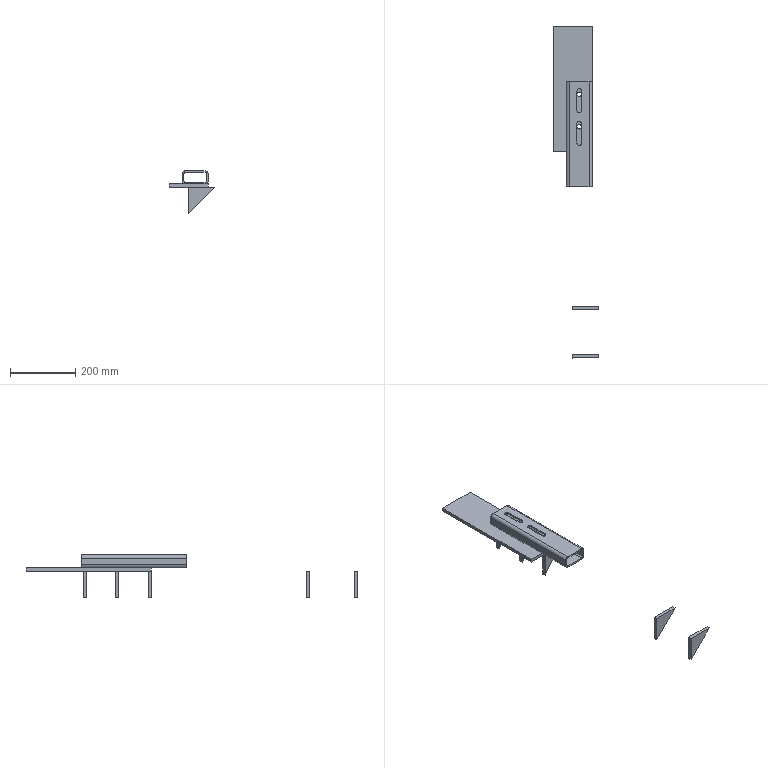Part | STEP file | rectangular upper-left upper why--2025.12.03 | 7 solids | 67 faces | box 140 x 1021 x 130.016 mm | volume 912623 mm3 | plane 49 | cylinder 18 | commonest cylinder face diameters 14 x10 10 x4 20 x4